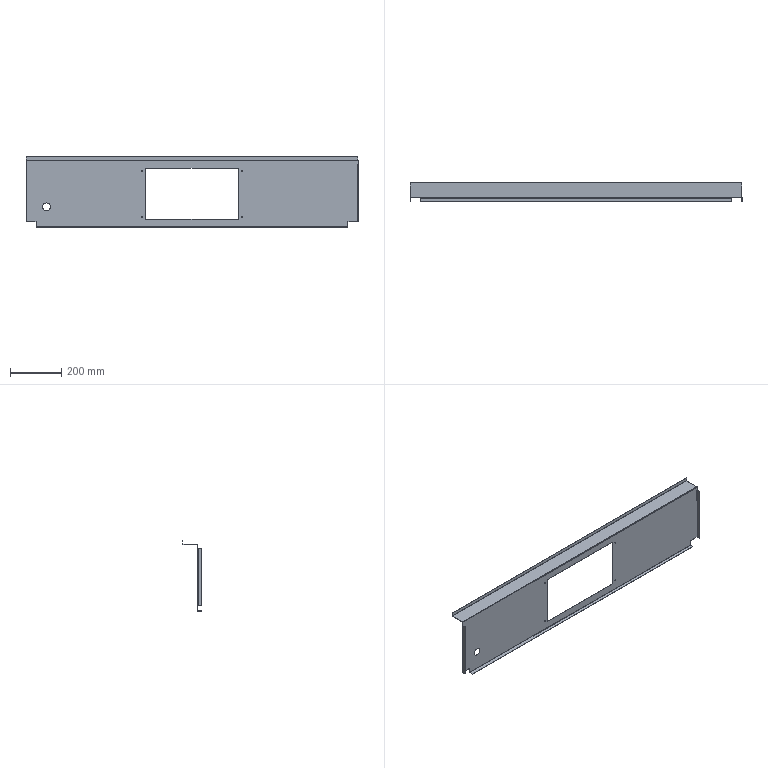Part | SolidWorks | features EdgeFlange 2, ICE 2, FlatPattern 1, SMBaseFlange 1, SheetMetal 1 | 1 solid | 64 faces | box 1298 x 73.8 x 275.3 mm | volume 455986 mm3 | plane 44 | cylinder 20 | commonest cylinder face diameters 4 x8 0.9 x5 3.3 x5 30 x2